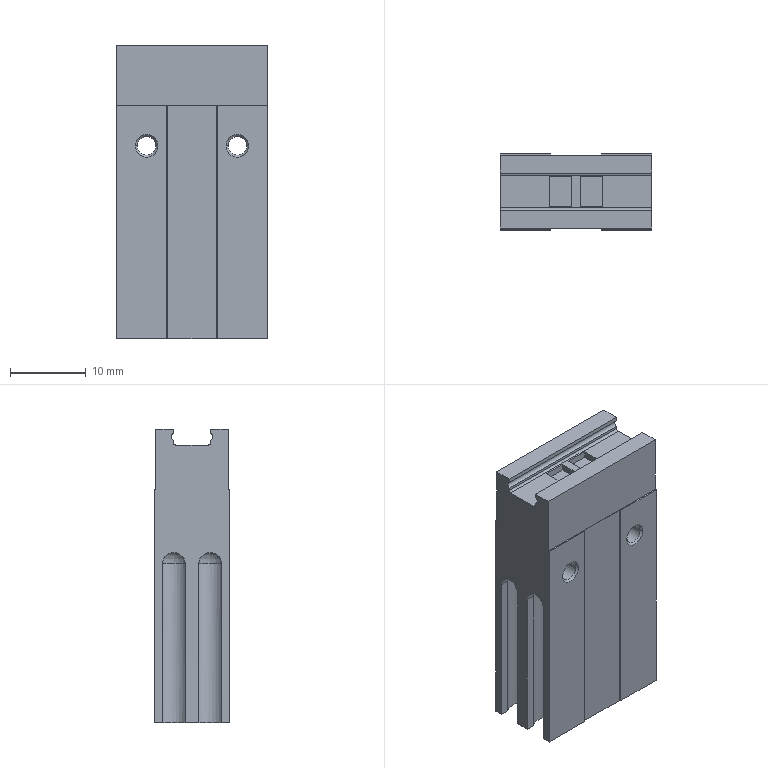Part | STEP file | MHZ2-6D2_Body(0).stp | 1 solid | 75 faces | box 20 x 10 x 38.8 mm | volume 6543 mm3 | plane 41 | cylinder 20 | cone 12 | sphere 2 | commonest cylinder face diameters 2.459 x8 3 x4 0.6 x2 1 x2 4 x2 7 x2